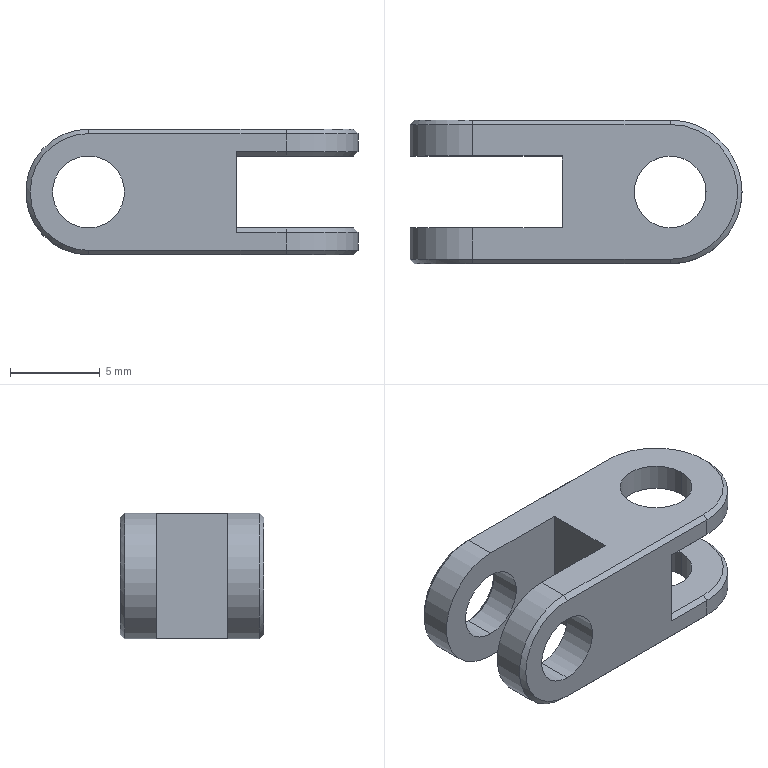Part | SolidWorks | features ICE 3, Chamfer 1, Extrusion 1, Scale 1 | 1 solid | 43 faces | box 18.5 x 8 x 7 mm | volume 447.364 mm3 | plane 19 | cylinder 14 | cone 10 | commonest cylinder face diameters 4 x8 8 x4 7 x2
STEP:
#1=CARTESIAN_POINT('',(14.75,4.,-3.5));
#2=VERTEX_POINT('',#1);
#3=CARTESIAN_POINT('',(11.,0.25,-3.5));
#4=VERTEX_POINT('',#3);
#5=CARTESIAN_POINT('',(11.,4.,-3.5));
#6=DIRECTION('',(0.,0.,-1.));
#7=DIRECTION('',(1.,0.,0.));
#8=AXIS2_PLACEMENT_3D('',#5,#6,#7);
#9=CIRCLE('',#8,3.75);
#10=EDGE_CURVE('',#2,#4,#9,.T.);
#11=ORIENTED_EDGE('',*,*,#10,.F.);
#12=CARTESIAN_POINT('',(15.,4.,-3.25));
#13=VERTEX_POINT('',#12);
#14=CARTESIAN_POINT('',(15.,4.,-3.25));
#15=DIRECTION('',(0.7071,0.,0.7071));
#16=VECTOR('',#15,1000.);
#17=LINE('',#14,#16);
#18=EDGE_CURVE('',#2,#13,#17,.T.);
#19=ORIENTED_EDGE('',*,*,#18,.T.);
#20=CARTESIAN_POINT('',(11.,0.,-3.25));
#21=VERTEX_POINT('',#20);
#22=CARTESIAN_POINT('',(11.,4.,-3.25));
#23=DIRECTION('',(0.,0.,1.));
#24=DIRECTION('',(1.,0.,0.));
#25=AXIS2_PLACEMENT_3D('',#22,#23,#24);
#26=CIRCLE('',#25,4.);
#27=EDGE_CURVE('',#21,#13,#26,.T.);
#28=ORIENTED_EDGE('',*,*,#27,.F.);
#29=CARTESIAN_POINT('',(11.,0.25,-3.5));
#30=DIRECTION('',(0.,-0.7071,0.7071));
#31=VECTOR('',#30,1000.);
#32=LINE('',#29,#31);
#33=EDGE_CURVE('',#4,#21,#32,.T.);
#34=ORIENTED_EDGE('',*,*,#33,.F.);
#35=EDGE_LOOP('',(#11,#19,#28,#34));
#36=FACE_OUTER_BOUND('',#35,.T.);
#37=CARTESIAN_POINT('',(11.,4.,-3.25));
#38=DIRECTION('',(0.,0.,1.));
#39=DIRECTION('',(1.,0.,0.));
#40=AXIS2_PLACEMENT_3D('',#37,#38,#39);
#41=CONICAL_SURFACE('',#40,4.,0.7854);
#42=ADVANCED_FACE('',(#36),#41,.T.);
#43=CARTESIAN_POINT('',(14.75,4.,2.));
#44=VERTEX_POINT('',#43);
#45=CARTESIAN_POINT('',(11.,0.25,2.));
#46=VERTEX_POINT('',#45);
#47=CARTESIAN_POINT('',(11.,4.,2.));
#48=DIRECTION('',(0.,0.,-1.));
#49=DIRECTION('',(1.,0.,0.));
#50=AXIS2_PLACEMENT_3D('',#47,#48,#49);
#51=CIRCLE('',#50,3.75);
#52=EDGE_CURVE('',#44,#46,#51,.T.);
#53=ORIENTED_EDGE('',*,*,#52,.F.);
#54=CARTESIAN_POINT('',(15.,4.,2.25));
#55=VERTEX_POINT('',#54);
#56=CARTESIAN_POINT('',(15.,4.,2.25));
#57=DIRECTION('',(0.7071,0.,0.7071));
#58=VECTOR('',#57,1000.);
#59=LINE('',#56,#58);
#60=EDGE_CURVE('',#44,#55,#59,.T.);
#61=ORIENTED_EDGE('',*,*,#60,.T.);
#62=CARTESIAN_POINT('',(11.,0.,2.25));
#63=VERTEX_POINT('',#62);
#64=CARTESIAN_POINT('',(11.,4.,2.25));
#65=DIRECTION('',(0.,0.,1.));
#66=DIRECTION('',(1.,0.,0.));
#67=AXIS2_PLACEMENT_3D('',#64,#65,#66);
#68=CIRCLE('',#67,4.);
#69=EDGE_CURVE('',#63,#55,#68,.T.);
#70=ORIENTED_EDGE('',*,*,#69,.F.);
#71=CARTESIAN_POINT('',(11.,0.,2.25));
#72=DIRECTION('',(0.,0.7071,-0.7071));
#73=VECTOR('',#72,1000.);
#74=LINE('',#71,#73);
#75=EDGE_CURVE('',#63,#46,#74,.T.);
#76=ORIENTED_EDGE('',*,*,#75,.T.);
#77=EDGE_LOOP('',(#53,#61,#70,#76));
#78=FACE_OUTER_BOUND('',#77,.T.);
#79=CARTESIAN_POINT('',(11.,4.,2.25));
#80=DIRECTION('',(0.,0.,1.));
#81=DIRECTION('',(1.,0.,0.));
#82=AXIS2_PLACEMENT_3D('',#79,#80,#81);
#83=CONICAL_SURFACE('',#82,4.,0.7854);
#84=ADVANCED_FACE('',(#78),#83,.T.);
#85=CARTESIAN_POINT('',(0.,7.75,-2.));
#86=VERTEX_POINT('',#85);
#87=CARTESIAN_POINT('',(0.,7.75,2.));
#88=VERTEX_POINT('',#87);
#89=CARTESIAN_POINT('',(0.,7.75,0.));
#90=DIRECTION('',(0.,1.,0.));
#91=DIRECTION('',(0.,0.,1.));
#92=AXIS2_PLACEMENT_3D('',#89,#90,#91);
#93=CIRCLE('',#92,2.);
#94=EDGE_CURVE('',#86,#88,#93,.T.);
#95=ORIENTED_EDGE('',*,*,#94,.F.);
#96=CARTESIAN_POINT('',(0.,8.,-2.25));
#97=VERTEX_POINT('',#96);
#98=CARTESIAN_POINT('',(0.,7.75,-2.));
#99=DIRECTION('',(0.,0.7071,-0.7071));
#100=VECTOR('',#99,1000.);
#101=LINE('',#98,#100);
#102=EDGE_CURVE('',#86,#97,#101,.T.);
#103=ORIENTED_EDGE('',*,*,#102,.T.);
#104=CARTESIAN_POINT('',(0.,8.,2.25));
#105=VERTEX_POINT('',#104);
#106=CARTESIAN_POINT('',(0.,8.,0.));
#107=DIRECTION('',(0.,-1.,0.));
#108=DIRECTION('',(0.,0.,1.));
#109=AXIS2_PLACEMENT_3D('',#106,#107,#108);
#110=CIRCLE('',#109,2.25);
#111=EDGE_CURVE('',#105,#97,#110,.T.);
#112=ORIENTED_EDGE('',*,*,#111,.F.);
#113=CARTESIAN_POINT('',(0.,7.75,2.));
#114=DIRECTION('',(0.,0.7071,0.7071));
#115=VECTOR('',#114,1000.);
#116=LINE('',#113,#115);
#117=EDGE_CURVE('',#88,#105,#116,.T.);
#118=ORIENTED_EDGE('',*,*,#117,.F.);
#119=EDGE_LOOP('',(#95,#103,#112,#118));
#120=FACE_OUTER_BOUND('',#119,.T.);
#121=CARTESIAN_POINT('',(0.,7.75,0.));
#122=DIRECTION('',(0.,1.,0.));
#123=DIRECTION('',(0.,0.,1.));
#124=AXIS2_PLACEMENT_3D('',#121,#122,#123);
#125=CONICAL_SURFACE('',#124,2.,0.7854);
#126=ADVANCED_FACE('',(#120),#125,.F.);
#127=CARTESIAN_POINT('',(9.,4.,2.));
#128=VERTEX_POINT('',#127);
#129=CARTESIAN_POINT('',(13.,4.,2.));
#130=VERTEX_POINT('',#129);
#131=CARTESIAN_POINT('',(11.,4.,2.));
#132=DIRECTION('',(0.,0.,1.));
#133=DIRECTION('',(1.,0.,0.));
#134=AXIS2_PLACEMENT_3D('',#131,#132,#133);
#135=CIRCLE('',#134,2.);
#136=EDGE_CURVE('',#128,#130,#135,.T.);
#137=ORIENTED_EDGE('',*,*,#136,.F.);
#138=CARTESIAN_POINT('',(9.,4.,3.5));
#139=VERTEX_POINT('',#138);
#140=CARTESIAN_POINT('',(9.,4.,-4.5));
#141=DIRECTION('',(0.,0.,1.));
#142=VECTOR('',#141,1000.);
#143=LINE('',#140,#142);
#144=EDGE_CURVE('',#128,#139,#143,.T.);
#145=ORIENTED_EDGE('',*,*,#144,.T.);
#146=CARTESIAN_POINT('',(13.,4.,3.5));
#147=VERTEX_POINT('',#146);
#148=CARTESIAN_POINT('',(11.,4.,3.5));
#149=DIRECTION('',(0.,0.,1.));
#150=DIRECTION('',(1.,0.,0.));
#151=AXIS2_PLACEMENT_3D('',#148,#149,#150);
#152=CIRCLE('',#151,2.);
#153=EDGE_CURVE('',#139,#147,#152,.T.);
#154=ORIENTED_EDGE('',*,*,#153,.T.);
#155=CARTESIAN_POINT('',(13.,4.,-4.5));
#156=DIRECTION('',(0.,0.,1.));
#157=VECTOR('',#156,1000.);
#158=LINE('',#155,#157);
#159=EDGE_CURVE('',#130,#147,#158,.T.);
#160=ORIENTED_EDGE('',*,*,#159,.F.);
#161=EDGE_LOOP('',(#137,#145,#154,#160));
#162=FACE_OUTER_BOUND('',#161,.T.);
#163=CARTESIAN_POINT('',(11.,4.,-4.5));
#164=DIRECTION('',(0.,0.,1.));
#165=DIRECTION('',(1.,0.,0.));
#166=AXIS2_PLACEMENT_3D('',#163,#164,#165);
#167=CYLINDRICAL_SURFACE('',#166,2.);
#168=ADVANCED_FACE('',(#162),#167,.F.);
#169=CARTESIAN_POINT('',(9.,4.,-3.5));
#170=VERTEX_POINT('',#169);
#171=CARTESIAN_POINT('',(13.,4.,-3.5));
#172=VERTEX_POINT('',#171);
#173=CARTESIAN_POINT('',(11.,4.,-3.5));
#174=DIRECTION('',(0.,0.,1.));
#175=DIRECTION('',(1.,0.,0.));
#176=AXIS2_PLACEMENT_3D('',#173,#174,#175);
#177=CIRCLE('',#176,2.);
#178=EDGE_CURVE('',#170,#172,#177,.T.);
#179=ORIENTED_EDGE('',*,*,#178,.F.);
#180=CARTESIAN_POINT('',(9.,4.,-2.));
#181=VERTEX_POINT('',#180);
#182=CARTESIAN_POINT('',(9.,4.,-4.5));
#183=DIRECTION('',(0.,0.,1.));
#184=VECTOR('',#183,1000.);
#185=LINE('',#182,#184);
#186=EDGE_CURVE('',#170,#181,#185,.T.);
#187=ORIENTED_EDGE('',*,*,#186,.T.);
#188=CARTESIAN_POINT('',(13.,4.,-2.));
#189=VERTEX_POINT('',#188);
#190=CARTESIAN_POINT('',(11.,4.,-2.));
#191=DIRECTION('',(0.,0.,-1.));
#192=DIRECTION('',(-1.,0.,0.));
#193=AXIS2_PLACEMENT_3D('',#190,#191,#192);
#194=CIRCLE('',#193,2.);
#195=EDGE_CURVE('',#189,#181,#194,.T.);
#196=ORIENTED_EDGE('',*,*,#195,.F.);
#197=CARTESIAN_POINT('',(13.,4.,-4.5));
#198=DIRECTION('',(0.,0.,1.));
#199=VECTOR('',#198,1000.);
#200=LINE('',#197,#199);
#201=EDGE_CURVE('',#172,#189,#200,.T.);
#202=ORIENTED_EDGE('',*,*,#201,.F.);
#203=EDGE_LOOP('',(#179,#187,#196,#202));
#204=FACE_OUTER_BOUND('',#203,.T.);
#205=CARTESIAN_POINT('',(11.,4.,-4.5));
#206=DIRECTION('',(0.,0.,1.));
#207=DIRECTION('',(1.,0.,0.));
#208=AXIS2_PLACEMENT_3D('',#205,#206,#207);
#209=CYLINDRICAL_SURFACE('',#208,2.);
#210=ADVANCED_FACE('',(#204),#209,.F.);
#211=ORIENTED_EDGE('',*,*,#69,.T.);
#212=CARTESIAN_POINT('',(15.,4.,3.25));
#213=VERTEX_POINT('',#212);
#214=CARTESIAN_POINT('',(15.,4.,-4.5));
#215=DIRECTION('',(0.,0.,1.));
#216=VECTOR('',#215,1000.);
#217=LINE('',#214,#216);
#218=EDGE_CURVE('',#55,#213,#217,.T.);
#219=ORIENTED_EDGE('',*,*,#218,.T.);
#220=CARTESIAN_POINT('',(11.,0.,3.25));
#221=VERTEX_POINT('',#220);
#222=CARTESIAN_POINT('',(11.,4.,3.25));
#223=DIRECTION('',(0.,0.,-1.));
#224=DIRECTION('',(-1.,0.,0.));
#225=AXIS2_PLACEMENT_3D('',#222,#223,#224);
#226=CIRCLE('',#225,4.);
#227=EDGE_CURVE('',#213,#221,#226,.T.);
#228=ORIENTED_EDGE('',*,*,#227,.T.);
#229=CARTESIAN_POINT('',(11.,0.,-4.5));
#230=DIRECTION('',(0.,0.,1.));
#231=VECTOR('',#230,1000.);
#232=LINE('',#229,#231);
#233=EDGE_CURVE('',#63,#221,#232,.T.);
#234=ORIENTED_EDGE('',*,*,#233,.F.);
#235=EDGE_LOOP('',(#211,#219,#228,#234));
#236=FACE_OUTER_BOUND('',#235,.T.);
#237=CARTESIAN_POINT('',(11.,4.,-4.5));
#238=DIRECTION('',(0.,0.,1.));
#239=DIRECTION('',(1.,0.,0.));
#240=AXIS2_PLACEMENT_3D('',#237,#238,#239);
#241=CYLINDRICAL_SURFACE('',#240,4.);
#242=ADVANCED_FACE('',(#236),#241,.T.);
#243=ORIENTED_EDGE('',*,*,#27,.T.);
#244=CARTESIAN_POINT('',(15.,4.,-2.25));
#245=VERTEX_POINT('',#244);
#246=CARTESIAN_POINT('',(15.,4.,-4.5));
#247=DIRECTION('',(0.,0.,1.));
#248=VECTOR('',#247,1000.);
#249=LINE('',#246,#248);
#250=EDGE_CURVE('',#13,#245,#249,.T.);
#251=ORIENTED_EDGE('',*,*,#250,.T.);
#252=CARTESIAN_POINT('',(11.,0.,-2.25));
#253=VERTEX_POINT('',#252);
#254=CARTESIAN_POINT('',(11.,4.,-2.25));
#255=DIRECTION('',(0.,0.,-1.));
#256=DIRECTION('',(-1.,0.,0.));
#257=AXIS2_PLACEMENT_3D('',#254,#255,#256);
#258=CIRCLE('',#257,4.);
#259=EDGE_CURVE('',#245,#253,#258,.T.);
#260=ORIENTED_EDGE('',*,*,#259,.T.);
#261=CARTESIAN_POINT('',(11.,0.,-4.5));
#262=DIRECTION('',(0.,0.,1.));
#263=VECTOR('',#262,1000.);
#264=LINE('',#261,#263);
#265=EDGE_CURVE('',#21,#253,#264,.T.);
#266=ORIENTED_EDGE('',*,*,#265,.F.);
#267=EDGE_LOOP('',(#243,#251,#260,#266));
#268=FACE_OUTER_BOUND('',#267,.T.);
#269=CARTESIAN_POINT('',(11.,4.,-4.5));
#270=DIRECTION('',(0.,0.,1.));
#271=DIRECTION('',(1.,0.,0.));
#272=AXIS2_PLACEMENT_3D('',#269,#270,#271);
#273=CYLINDRICAL_SURFACE('',#272,4.);
#274=ADVANCED_FACE('',(#268),#273,.T.);
#275=ORIENTED_EDGE('',*,*,#94,.T.);
#276=CARTESIAN_POINT('',(0.,6.,2.));
#277=VERTEX_POINT('',#276);
#278=CARTESIAN_POINT('',(0.,8.,2.));
#279=DIRECTION('',(0.,-1.,0.));
#280=VECTOR('',#279,1000.);
#281=LINE('',#278,#280);
#282=EDGE_CURVE('',#88,#277,#281,.T.);
#283=ORIENTED_EDGE('',*,*,#282,.T.);
#284=CARTESIAN_POINT('',(0.,6.,-2.));
#285=VERTEX_POINT('',#284);
#286=CARTESIAN_POINT('',(0.,6.,0.));
#287=DIRECTION('',(0.,-1.,0.));
#288=DIRECTION('',(0.,0.,-1.));
#289=AXIS2_PLACEMENT_3D('',#286,#287,#288);
#290=CIRCLE('',#289,2.);
#291=EDGE_CURVE('',#277,#285,#290,.T.);
#292=ORIENTED_EDGE('',*,*,#291,.T.);
#293=CARTESIAN_POINT('',(0.,8.,-2.));
#294=DIRECTION('',(0.,-1.,0.));
#295=VECTOR('',#294,1000.);
#296=LINE('',#293,#295);
#297=EDGE_CURVE('',#86,#285,#296,.T.);
#298=ORIENTED_EDGE('',*,*,#297,.F.);
#299=EDGE_LOOP('',(#275,#283,#292,#298));
#300=FACE_OUTER_BOUND('',#299,.T.);
#301=CARTESIAN_POINT('',(0.,8.,0.));
#302=DIRECTION('',(0.,-1.,0.));
#303=DIRECTION('',(0.,0.,-1.));
#304=AXIS2_PLACEMENT_3D('',#301,#302,#303);
#305=CYLINDRICAL_SURFACE('',#304,2.);
#306=ADVANCED_FACE('',(#300),#305,.F.);
#307=CARTESIAN_POINT('',(0.,2.,-2.));
#308=VERTEX_POINT('',#307);
#309=CARTESIAN_POINT('',(0.,2.,2.));
#310=VERTEX_POINT('',#309);
#311=CARTESIAN_POINT('',(0.,2.,0.));
#312=DIRECTION('',(0.,1.,0.));
#313=DIRECTION('',(0.,0.,1.));
#314=AXIS2_PLACEMENT_3D('',#311,#312,#313);
#315=CIRCLE('',#314,2.);
#316=EDGE_CURVE('',#308,#310,#315,.T.);
#317=ORIENTED_EDGE('',*,*,#316,.T.);
#318=CARTESIAN_POINT('',(0.,0.,2.));
#319=VERTEX_POINT('',#318);
#320=CARTESIAN_POINT('',(0.,8.,2.));
#321=DIRECTION('',(0.,-1.,0.));
#322=VECTOR('',#321,1000.);
#323=LINE('',#320,#322);
#324=EDGE_CURVE('',#310,#319,#323,.T.);
#325=ORIENTED_EDGE('',*,*,#324,.T.);
#326=CARTESIAN_POINT('',(0.,0.,-2.));
#327=VERTEX_POINT('',#326);
#328=CARTESIAN_POINT('',(0.,0.,0.));
#329=DIRECTION('',(0.,1.,0.));
#330=DIRECTION('',(0.,0.,1.));
#331=AXIS2_PLACEMENT_3D('',#328,#329,#330);
#332=CIRCLE('',#331,2.);
#333=EDGE_CURVE('',#327,#319,#332,.T.);
#334=ORIENTED_EDGE('',*,*,#333,.F.);
#335=CARTESIAN_POINT('',(0.,8.,-2.));
#336=DIRECTION('',(0.,-1.,0.));
#337=VECTOR('',#336,1000.);
#338=LINE('',#335,#337);
#339=EDGE_CURVE('',#308,#327,#338,.T.);
#340=ORIENTED_EDGE('',*,*,#339,.F.);
#341=EDGE_LOOP('',(#317,#325,#334,#340));
#342=FACE_OUTER_BOUND('',#341,.T.);
#343=CARTESIAN_POINT('',(0.,8.,0.));
#344=DIRECTION('',(0.,-1.,0.));
#345=DIRECTION('',(0.,0.,-1.));
#346=AXIS2_PLACEMENT_3D('',#343,#344,#345);
#347=CYLINDRICAL_SURFACE('',#346,2.);
#348=ADVANCED_FACE('',(#342),#347,.F.);
#349=CARTESIAN_POINT('',(11.,4.,3.5));
#350=DIRECTION('',(0.,0.,1.));
#351=DIRECTION('',(1.,0.,0.));
#352=AXIS2_PLACEMENT_3D('',#349,#350,#351);
#353=CIRCLE('',#352,2.);
#354=EDGE_CURVE('',#147,#139,#353,.T.);
#355=ORIENTED_EDGE('',*,*,#354,.F.);
#356=ORIENTED_EDGE('',*,*,#153,.F.);
#357=EDGE_LOOP('',(#355,#356));
#358=FACE_BOUND('',#357,.T.);
#359=CARTESIAN_POINT('',(0.,2.,3.5));
#360=VERTEX_POINT('',#359);
#361=CARTESIAN_POINT('',(0.,0.25,3.5));
#362=VERTEX_POINT('',#361);
#363=CARTESIAN_POINT('',(0.,8.,3.5));
#364=DIRECTION('',(0.,-1.,0.));
#365=VECTOR('',#364,1000.);
#366=LINE('',#363,#365);
#367=EDGE_CURVE('',#360,#362,#366,.T.);
#368=ORIENTED_EDGE('',*,*,#367,.T.);
#369=CARTESIAN_POINT('',(11.,0.25,3.5));
#370=VERTEX_POINT('',#369);
#371=CARTESIAN_POINT('',(0.,0.25,3.5));
#372=DIRECTION('',(1.,0.,0.));
#373=VECTOR('',#372,1000.);
#374=LINE('',#371,#373);
#375=EDGE_CURVE('',#362,#370,#374,.T.);
#376=ORIENTED_EDGE('',*,*,#375,.T.);
#377=CARTESIAN_POINT('',(11.,7.75,3.5));
#378=VERTEX_POINT('',#377);
#379=CARTESIAN_POINT('',(11.,4.,3.5));
#380=DIRECTION('',(0.,0.,1.));
#381=DIRECTION('',(-1.,0.,0.));
#382=AXIS2_PLACEMENT_3D('',#379,#380,#381);
#383=CIRCLE('',#382,3.75);
#384=EDGE_CURVE('',#370,#378,#383,.T.);
#385=ORIENTED_EDGE('',*,*,#384,.T.);
#386=CARTESIAN_POINT('',(0.,7.75,3.5));
#387=VERTEX_POINT('',#386);
#388=CARTESIAN_POINT('',(0.,7.75,3.5));
#389=DIRECTION('',(-1.,0.,0.));
#390=VECTOR('',#389,1000.);
#391=LINE('',#388,#390);
#392=EDGE_CURVE('',#378,#387,#391,.T.);
#393=ORIENTED_EDGE('',*,*,#392,.T.);
#394=CARTESIAN_POINT('',(0.,6.,3.5));
#395=VERTEX_POINT('',#394);
#396=CARTESIAN_POINT('',(0.,8.,3.5));
#397=DIRECTION('',(0.,-1.,0.));
#398=VECTOR('',#397,1000.);
#399=LINE('',#396,#398);
#400=EDGE_CURVE('',#387,#395,#399,.T.);
#401=ORIENTED_EDGE('',*,*,#400,.T.);
#402=CARTESIAN_POINT('',(5.,6.,3.5));
#403=VERTEX_POINT('',#402);
#404=CARTESIAN_POINT('',(5.,6.,3.5));
#405=DIRECTION('',(-1.,0.,0.));
#406=VECTOR('',#405,1000.);
#407=LINE('',#404,#406);
#408=EDGE_CURVE('',#403,#395,#407,.T.);
#409=ORIENTED_EDGE('',*,*,#408,.F.);
#410=CARTESIAN_POINT('',(5.,2.,3.5));
#411=VERTEX_POINT('',#410);
#412=CARTESIAN_POINT('',(5.,6.,3.5));
#413=DIRECTION('',(0.,-1.,0.));
#414=VECTOR('',#413,1000.);
#415=LINE('',#412,#414);
#416=EDGE_CURVE('',#403,#411,#415,.T.);
#417=ORIENTED_EDGE('',*,*,#416,.T.);
#418=CARTESIAN_POINT('',(5.,2.,3.5));
#419=DIRECTION('',(-1.,0.,0.));
#420=VECTOR('',#419,1000.);
#421=LINE('',#418,#420);
#422=EDGE_CURVE('',#411,#360,#421,.T.);
#423=ORIENTED_EDGE('',*,*,#422,.T.);
#424=EDGE_LOOP('',(#368,#376,#385,#393,#401,#409,#417,#423));
#425=FACE_OUTER_BOUND('',#424,.T.);
#426=CARTESIAN_POINT('',(0.,8.,3.5));
#427=DIRECTION('',(0.,0.,-1.));
#428=DIRECTION('',(-1.,0.,0.));
#429=AXIS2_PLACEMENT_3D('',#426,#427,#428);
#430=PLANE('',#429);
#431=ADVANCED_FACE('',(#358,#425),#430,.F.);
#432=CARTESIAN_POINT('',(11.,4.,-3.5));
#433=DIRECTION('',(0.,0.,1.));
#434=DIRECTION('',(1.,0.,0.));
#435=AXIS2_PLACEMENT_3D('',#432,#433,#434);
#436=CIRCLE('',#435,2.);
#437=EDGE_CURVE('',#172,#170,#436,.T.);
#438=ORIENTED_EDGE('',*,*,#437,.T.);
#439=ORIENTED_EDGE('',*,*,#178,.T.);
#440=EDGE_LOOP('',(#438,#439));
#441=FACE_BOUND('',#440,.T.);
#442=CARTESIAN_POINT('',(11.,7.75,-3.5));
#443=VERTEX_POINT('',#442);
#444=CARTESIAN_POINT('',(11.,4.,-3.5));
#445=DIRECTION('',(0.,0.,-1.));
#446=DIRECTION('',(1.,0.,0.));
#447=AXIS2_PLACEMENT_3D('',#444,#445,#446);
#448=CIRCLE('',#447,3.75);
#449=EDGE_CURVE('',#443,#2,#448,.T.);
#450=ORIENTED_EDGE('',*,*,#449,.T.);
#451=ORIENTED_EDGE('',*,*,#10,.T.);
#452=CARTESIAN_POINT('',(0.,0.25,-3.5));
#453=VERTEX_POINT('',#452);
#454=CARTESIAN_POINT('',(0.,0.25,-3.5));
#455=DIRECTION('',(-1.,0.,0.));
#456=VECTOR('',#455,1000.);
#457=LINE('',#454,#456);
#458=EDGE_CURVE('',#4,#453,#457,.T.);
#459=ORIENTED_EDGE('',*,*,#458,.T.);
#460=CARTESIAN_POINT('',(0.,2.,-3.5));
#461=VERTEX_POINT('',#460);
#462=CARTESIAN_POINT('',(0.,8.,-3.5));
#463=DIRECTION('',(0.,-1.,0.));
#464=VECTOR('',#463,1000.);
#465=LINE('',#462,#464);
#466=EDGE_CURVE('',#461,#453,#465,.T.);
#467=ORIENTED_EDGE('',*,*,#466,.F.);
#468=CARTESIAN_POINT('',(5.,2.,-3.5));
#469=VERTEX_POINT('',#468);
#470=CARTESIAN_POINT('',(5.,2.,-3.5));
#471=DIRECTION('',(-1.,0.,0.));
#472=VECTOR('',#471,1000.);
#473=LINE('',#470,#472);
#474=EDGE_CURVE('',#469,#461,#473,.T.);
#475=ORIENTED_EDGE('',*,*,#474,.F.);
#476=CARTESIAN_POINT('',(5.,6.,-3.5));
#477=VERTEX_POINT('',#476);
#478=CARTESIAN_POINT('',(5.,6.,-3.5));
#479=DIRECTION('',(0.,1.,0.));
#480=VECTOR('',#479,1000.);
#481=LINE('',#478,#480);
#482=EDGE_CURVE('',#469,#477,#481,.T.);
#483=ORIENTED_EDGE('',*,*,#482,.T.);
#484=CARTESIAN_POINT('',(0.,6.,-3.5));
#485=VERTEX_POINT('',#484);
#486=CARTESIAN_POINT('',(5.,6.,-3.5));
#487=DIRECTION('',(-1.,0.,0.));
#488=VECTOR('',#487,1000.);
#489=LINE('',#486,#488);
#490=EDGE_CURVE('',#477,#485,#489,.T.);
#491=ORIENTED_EDGE('',*,*,#490,.T.);
#492=CARTESIAN_POINT('',(0.,7.75,-3.5));
#493=VERTEX_POINT('',#492);
#494=CARTESIAN_POINT('',(0.,8.,-3.5));
#495=DIRECTION('',(0.,-1.,0.));
#496=VECTOR('',#495,1000.);
#497=LINE('',#494,#496);
#498=EDGE_CURVE('',#493,#485,#497,.T.);
#499=ORIENTED_EDGE('',*,*,#498,.F.);
#500=CARTESIAN_POINT('',(11.,7.75,-3.5));
#501=DIRECTION('',(1.,0.,0.));
#502=VECTOR('',#501,1000.);
#503=LINE('',#500,#502);
#504=EDGE_CURVE('',#493,#443,#503,.T.);
#505=ORIENTED_EDGE('',*,*,#504,.T.);
#506=EDGE_LOOP('',(#450,#451,#459,#467,#475,#483,#491,#499,#505));
#507=FACE_OUTER_BOUND('',#506,.T.);
#508=CARTESIAN_POINT('',(0.,8.,-3.5));
#509=DIRECTION('',(0.,0.,1.));
#510=DIRECTION('',(1.,0.,0.));
#511=AXIS2_PLACEMENT_3D('',#508,#509,#510);
#512=PLANE('',#511);
#513=ADVANCED_FACE('',(#441,#507),#512,.F.);
#514=ORIENTED_EDGE('',*,*,#466,.T.);
#515=CARTESIAN_POINT('',(0.,0.25,0.));
#516=DIRECTION('',(0.,1.,0.));
#517=DIRECTION('',(0.,0.,1.));
#518=AXIS2_PLACEMENT_3D('',#515,#516,#517);
#519=CIRCLE('',#518,3.5);
#520=EDGE_CURVE('',#453,#362,#519,.T.);
#521=ORIENTED_EDGE('',*,*,#520,.T.);
#522=ORIENTED_EDGE('',*,*,#367,.F.);
#523=CARTESIAN_POINT('',(0.,2.,0.));
#524=DIRECTION('',(0.,1.,0.));
#525=DIRECTION('',(0.,0.,1.));
#526=AXIS2_PLACEMENT_3D('',#523,#524,#525);
#527=CIRCLE('',#526,3.5);
#528=EDGE_CURVE('',#461,#360,#527,.T.);
#529=ORIENTED_EDGE('',*,*,#528,.F.);
#530=EDGE_LOOP('',(#514,#521,#522,#529));
#531=FACE_OUTER_BOUND('',#530,.T.);
#532=CARTESIAN_POINT('',(0.,8.,0.));
#533=DIRECTION('',(0.,-1.,0.));
#534=DIRECTION('',(0.,0.,-1.));
#535=AXIS2_PLACEMENT_3D('',#532,#533,#534);
#536=CYLINDRICAL_SURFACE('',#535,3.5);
#537=ADVANCED_FACE('',(#531),#536,.T.);
#538=ORIENTED_EDGE('',*,*,#400,.F.);
#539=CARTESIAN_POINT('',(0.,7.75,0.));
#540=DIRECTION('',(0.,-1.,0.));
#541=DIRECTION('',(0.,0.,1.));
#542=AXIS2_PLACEMENT_3D('',#539,#540,#541);
#543=CIRCLE('',#542,3.5);
#544=EDGE_CURVE('',#387,#493,#543,.T.);
#545=ORIENTED_EDGE('',*,*,#544,.T.);
#546=ORIENTED_EDGE('',*,*,#498,.T.);
#547=CARTESIAN_POINT('',(0.,6.,0.));
#548=DIRECTION('',(0.,-1.,0.));
#549=DIRECTION('',(0.,0.,-1.));
#550=AXIS2_PLACEMENT_3D('',#547,#548,#549);
#551=CIRCLE('',#550,3.5);
#552=EDGE_CURVE('',#395,#485,#551,.T.);
#553=ORIENTED_EDGE('',*,*,#552,.F.);
#554=EDGE_LOOP('',(#538,#545,#546,#553));
#555=FACE_OUTER_BOUND('',#554,.T.);
#556=CARTESIAN_POINT('',(0.,8.,0.));
#557=DIRECTION('',(0.,-1.,0.));
#558=DIRECTION('',(0.,0.,-1.));
#559=AXIS2_PLACEMENT_3D('',#556,#557,#558);
#560=CYLINDRICAL_SURFACE('',#559,3.5);
#561=ADVANCED_FACE('',(#555),#560,.T.);
#562=ORIENTED_EDGE('',*,*,#324,.F.);
#563=CARTESIAN_POINT('',(0.,2.,0.));
#564=DIRECTION('',(0.,1.,0.));
#565=DIRECTION('',(0.,0.,1.));
#566=AXIS2_PLACEMENT_3D('',#563,#564,#565);
#567=CIRCLE('',#566,2.);
#568=EDGE_CURVE('',#310,#308,#567,.T.);
#569=ORIENTED_EDGE('',*,*,#568,.T.);
#570=ORIENTED_EDGE('',*,*,#339,.T.);
#571=CARTESIAN_POINT('',(0.,0.,0.));
#572=DIRECTION('',(0.,1.,0.));
#573=DIRECTION('',(0.,0.,1.));
#574=AXIS2_PLACEMENT_3D('',#571,#572,#573);
#575=CIRCLE('',#574,2.);
#576=EDGE_CURVE('',#319,#327,#575,.T.);
#577=ORIENTED_EDGE('',*,*,#576,.F.);
#578=EDGE_LOOP('',(#562,#569,#570,#577));
#579=FACE_OUTER_BOUND('',#578,.T.);
#580=CARTESIAN_POINT('',(0.,8.,0.));
#581=DIRECTION('',(0.,-1.,0.));
#582=DIRECTION('',(0.,0.,-1.));
#583=AXIS2_PLACEMENT_3D('',#580,#581,#582);
#584=CYLINDRICAL_SURFACE('',#583,2.);
#585=ADVANCED_FACE('',(#579),#584,.F.);
#586=ORIENTED_EDGE('',*,*,#282,.F.);
#587=CARTESIAN_POINT('',(0.,7.75,0.));
#588=DIRECTION('',(0.,1.,0.));
#589=DIRECTION('',(0.,0.,1.));
#590=AXIS2_PLACEMENT_3D('',#587,#588,#589);
#591=CIRCLE('',#590,2.);
#592=EDGE_CURVE('',#88,#86,#591,.T.);
#593=ORIENTED_EDGE('',*,*,#592,.T.);
#594=ORIENTED_EDGE('',*,*,#297,.T.);
#595=CARTESIAN_POINT('',(0.,6.,0.));
#596=DIRECTION('',(0.,-1.,0.));
#597=DIRECTION('',(0.,0.,-1.));
#598=AXIS2_PLACEMENT_3D('',#595,#596,#597);
#599=CIRCLE('',#598,2.);
#600=EDGE_CURVE('',#285,#277,#599,.T.);
#601=ORIENTED_EDGE('',*,*,#600,.T.);
#602=EDGE_LOOP('',(#586,#593,#594,#601));
#603=FACE_OUTER_BOUND('',#602,.T.);
#604=CARTESIAN_POINT('',(0.,8.,0.));
#605=DIRECTION('',(0.,-1.,0.));
#606=DIRECTION('',(0.,0.,-1.));
#607=AXIS2_PLACEMENT_3D('',#604,#605,#606);
#608=CYLINDRICAL_SURFACE('',#607,2.);
#609=ADVANCED_FACE('',(#603),#608,.F.);
#610=CARTESIAN_POINT('',(11.,4.,2.));
#611=DIRECTION('',(0.,0.,1.));
#612=DIRECTION('',(1.,0.,0.));
#613=AXIS2_PLACEMENT_3D('',#610,#611,#612);
#614=CIRCLE('',#613,2.);
#615=EDGE_CURVE('',#130,#128,#614,.T.);
#616=ORIENTED_EDGE('',*,*,#615,.T.);
#617=ORIENTED_EDGE('',*,*,#136,.T.);
#618=EDGE_LOOP('',(#616,#617));
#619=FACE_BOUND('',#618,.T.);
#620=CARTESIAN_POINT('',(11.,7.75,2.));
#621=VERTEX_POINT('',#620);
#622=CARTESIAN_POINT('',(11.,4.,2.));
#623=DIRECTION('',(0.,0.,-1.));
#624=DIRECTION('',(1.,0.,0.));
#625=AXIS2_PLACEMENT_3D('',#622,#623,#624);
#626=CIRCLE('',#625,3.75);
#627=EDGE_CURVE('',#621,#44,#626,.T.);
#628=ORIENTED_EDGE('',*,*,#627,.T.);
#629=ORIENTED_EDGE('',*,*,#52,.T.);
#630=CARTESIAN_POINT('',(8.232,0.25,2.));
#631=VERTEX_POINT('',#630);
#632=CARTESIAN_POINT('',(15.,0.25,2.));
#633=DIRECTION('',(-1.,0.,0.));
#634=VECTOR('',#633,1000.);
#635=LINE('',#632,#634);
#636=EDGE_CURVE('',#46,#631,#635,.T.);
#637=ORIENTED_EDGE('',*,*,#636,.T.);
#638=CARTESIAN_POINT('',(8.232,7.75,2.));
#639=VERTEX_POINT('',#638);
#640=CARTESIAN_POINT('',(8.232,0.,2.));
#641=DIRECTION('',(0.,1.,0.));
#642=VECTOR('',#641,1000.);
#643=LINE('',#640,#642);
#644=EDGE_CURVE('',#631,#639,#643,.T.);
#645=ORIENTED_EDGE('',*,*,#644,.T.);
#646=CARTESIAN_POINT('',(11.,7.75,2.));
#647=DIRECTION('',(1.,0.,0.));
#648=VECTOR('',#647,1000.);
#649=LINE('',#646,#648);
#650=EDGE_CURVE('',#639,#621,#649,.T.);
#651=ORIENTED_EDGE('',*,*,#650,.T.);
#652=EDGE_LOOP('',(#628,#629,#637,#645,#651));
#653=FACE_OUTER_BOUND('',#652,.T.);
#654=CARTESIAN_POINT('',(15.,0.,2.));
#655=DIRECTION('',(0.,0.,1.));
#656=DIRECTION('',(1.,0.,0.));
#657=AXIS2_PLACEMENT_3D('',#654,#655,#656);
#658=PLANE('',#657);
#659=ADVANCED_FACE('',(#619,#653),#658,.F.);
#660=ORIENTED_EDGE('',*,*,#195,.T.);
#661=CARTESIAN_POINT('',(11.,4.,-2.));
#662=DIRECTION('',(0.,0.,-1.));
#663=DIRECTION('',(-1.,0.,0.));
#664=AXIS2_PLACEMENT_3D('',#661,#662,#663);
#665=CIRCLE('',#664,2.);
#666=EDGE_CURVE('',#181,#189,#665,.T.);
#667=ORIENTED_EDGE('',*,*,#666,.T.);
#668=EDGE_LOOP('',(#660,#667));
#669=FACE_BOUND('',#668,.T.);
#670=CARTESIAN_POINT('',(8.232,0.25,-2.));
#671=VERTEX_POINT('',#670);
#672=CARTESIAN_POINT('',(8.232,7.75,-2.));
#673=VERTEX_POINT('',#672);
#674=CARTESIAN_POINT('',(8.232,0.,-2.));
#675=DIRECTION('',(0.,1.,0.));
#676=VECTOR('',#675,1000.);
#677=LINE('',#674,#676);
#678=EDGE_CURVE('',#671,#673,#677,.T.);
#679=ORIENTED_EDGE('',*,*,#678,.F.);
#680=CARTESIAN_POINT('',(11.,0.25,-2.));
#681=VERTEX_POINT('',#680);
#682=CARTESIAN_POINT('',(15.,0.25,-2.));
#683=DIRECTION('',(1.,0.,0.));
#684=VECTOR('',#683,1000.);
#685=LINE('',#682,#684);
#686=EDGE_CURVE('',#671,#681,#685,.T.);
#687=ORIENTED_EDGE('',*,*,#686,.T.);
#688=CARTESIAN_POINT('',(11.,7.75,-2.));
#689=VERTEX_POINT('',#688);
#690=CARTESIAN_POINT('',(11.,4.,-2.));
#691=DIRECTION('',(0.,0.,1.));
#692=DIRECTION('',(-1.,0.,0.));
#693=AXIS2_PLACEMENT_3D('',#690,#691,#692);
#694=CIRCLE('',#693,3.75);
#695=EDGE_CURVE('',#681,#689,#694,.T.);
#696=ORIENTED_EDGE('',*,*,#695,.T.);
#697=CARTESIAN_POINT('',(8.232,7.75,-2.));
#698=DIRECTION('',(-1.,0.,0.));
#699=VECTOR('',#698,1000.);
#700=LINE('',#697,#699);
#701=EDGE_CURVE('',#689,#673,#700,.T.);
#702=ORIENTED_EDGE('',*,*,#701,.T.);
#703=EDGE_LOOP('',(#679,#687,#696,#702));
#704=FACE_OUTER_BOUND('',#703,.T.);
#705=CARTESIAN_POINT('',(15.,0.,-2.));
#706=DIRECTION('',(0.,0.,-1.));
#707=DIRECTION('',(-1.,0.,0.));
#708=AXIS2_PLACEMENT_3D('',#705,#706,#707);
#709=PLANE('',#708);
#710=ADVANCED_FACE('',(#669,#704),#709,.F.);
#711=ORIENTED_EDGE('',*,*,#111,.T.);
#712=CARTESIAN_POINT('',(0.,8.,0.));
#713=DIRECTION('',(0.,-1.,0.));
#714=DIRECTION('',(0.,0.,1.));
#715=AXIS2_PLACEMENT_3D('',#712,#713,#714);
#716=CIRCLE('',#715,2.25);
#717=EDGE_CURVE('',#97,#105,#716,.T.);
#718=ORIENTED_EDGE('',*,*,#717,.T.);
#719=EDGE_LOOP('',(#711,#718));
#720=FACE_BOUND('',#719,.T.);
#721=CARTESIAN_POINT('',(7.982,8.,2.25));
#722=VERTEX_POINT('',#721);
#723=CARTESIAN_POINT('',(7.982,8.,-2.25));
#724=VERTEX_POINT('',#723);
#725=CARTESIAN_POINT('',(7.982,8.,-2.));
#726=DIRECTION('',(0.,0.,-1.));
#727=VECTOR('',#726,1000.);
#728=LINE('',#725,#727);
#729=EDGE_CURVE('',#722,#724,#728,.T.);
#730=ORIENTED_EDGE('',*,*,#729,.T.);
#731=CARTESIAN_POINT('',(11.,8.,-2.25));
#732=VERTEX_POINT('',#731);
#733=CARTESIAN_POINT('',(11.,8.,-2.25));
#734=DIRECTION('',(1.,0.,0.));
#735=VECTOR('',#734,1000.);
#736=LINE('',#733,#735);
#737=EDGE_CURVE('',#724,#732,#736,.T.);
#738=ORIENTED_EDGE('',*,*,#737,.T.);
#739=CARTESIAN_POINT('',(11.,8.,-3.25));
#740=VERTEX_POINT('',#739);
#741=CARTESIAN_POINT('',(11.,8.,-4.5));
#742=DIRECTION('',(0.,0.,1.));
#743=VECTOR('',#742,1000.);
#744=LINE('',#741,#743);
#745=EDGE_CURVE('',#740,#732,#744,.T.);
#746=ORIENTED_EDGE('',*,*,#745,.F.);
#747=CARTESIAN_POINT('',(0.,8.,-3.25));
#748=VERTEX_POINT('',#747);
#749=CARTESIAN_POINT('',(0.,8.,-3.25));
#750=DIRECTION('',(-1.,0.,0.));
#751=VECTOR('',#750,1000.);
#752=LINE('',#749,#751);
#753=EDGE_CURVE('',#740,#748,#752,.T.);
#754=ORIENTED_EDGE('',*,*,#753,.T.);
#755=CARTESIAN_POINT('',(0.,8.,3.25));
#756=VERTEX_POINT('',#755);
#757=CARTESIAN_POINT('',(0.,8.,0.));
#758=DIRECTION('',(0.,1.,0.));
#759=DIRECTION('',(0.,0.,1.));
#760=AXIS2_PLACEMENT_3D('',#757,#758,#759);
#761=CIRCLE('',#760,3.25);
#762=EDGE_CURVE('',#748,#756,#761,.T.);
#763=ORIENTED_EDGE('',*,*,#762,.T.);
#764=CARTESIAN_POINT('',(11.,8.,3.25));
#765=VERTEX_POINT('',#764);
#766=CARTESIAN_POINT('',(11.,8.,3.25));
#767=DIRECTION('',(1.,0.,0.));
#768=VECTOR('',#767,1000.);
#769=LINE('',#766,#768);
#770=EDGE_CURVE('',#756,#765,#769,.T.);
#771=ORIENTED_EDGE('',*,*,#770,.T.);
#772=CARTESIAN_POINT('',(11.,8.,2.25));
#773=VERTEX_POINT('',#772);
#774=CARTESIAN_POINT('',(11.,8.,-4.5));
#775=DIRECTION('',(0.,0.,1.));
#776=VECTOR('',#775,1000.);
#777=LINE('',#774,#776);
#778=EDGE_CURVE('',#773,#765,#777,.T.);
#779=ORIENTED_EDGE('',*,*,#778,.F.);
#780=CARTESIAN_POINT('',(8.232,8.,2.25));
#781=DIRECTION('',(-1.,0.,0.));
#782=VECTOR('',#781,1000.);
#783=LINE('',#780,#782);
#784=EDGE_CURVE('',#773,#722,#783,.T.);
#785=ORIENTED_EDGE('',*,*,#784,.T.);
#786=EDGE_LOOP('',(#730,#738,#746,#754,#763,#771,#779,#785));
#787=FACE_OUTER_BOUND('',#786,.T.);
#788=CARTESIAN_POINT('',(0.,8.,0.));
#789=DIRECTION('',(0.,1.,0.));
#790=DIRECTION('',(0.,0.,1.));
#791=AXIS2_PLACEMENT_3D('',#788,#789,#790);
#792=PLANE('',#791);
#793=ADVANCED_FACE('',(#720,#787),#792,.T.);
#794=ORIENTED_EDGE('',*,*,#265,.T.);
#795=CARTESIAN_POINT('',(8.232,0.,-2.25));
#796=VERTEX_POINT('',#795);
#797=CARTESIAN_POINT('',(0.,0.,-2.25));
#798=DIRECTION('',(-1.,0.,0.));
#799=VECTOR('',#798,1000.);
#800=LINE('',#797,#799);
#801=EDGE_CURVE('',#253,#796,#800,.T.);
#802=ORIENTED_EDGE('',*,*,#801,.T.);
#803=CARTESIAN_POINT('',(8.232,0.,2.25));
#804=VERTEX_POINT('',#803);
#805=CARTESIAN_POINT('',(8.232,0.,-2.));
#806=DIRECTION('',(0.,0.,1.));
#807=VECTOR('',#806,1000.);
#808=LINE('',#805,#807);
#809=EDGE_CURVE('',#796,#804,#808,.T.);
#810=ORIENTED_EDGE('',*,*,#809,.T.);
#811=CARTESIAN_POINT('',(0.,0.,2.25));
#812=DIRECTION('',(1.,0.,0.));
#813=VECTOR('',#812,1000.);
#814=LINE('',#811,#813);
#815=EDGE_CURVE('',#804,#63,#814,.T.);
#816=ORIENTED_EDGE('',*,*,#815,.T.);
#817=ORIENTED_EDGE('',*,*,#233,.T.);
#818=CARTESIAN_POINT('',(0.,0.,3.25));
#819=VERTEX_POINT('',#818);
#820=CARTESIAN_POINT('',(0.,0.,3.25));
#821=DIRECTION('',(-1.,0.,0.));
#822=VECTOR('',#821,1000.);
#823=LINE('',#820,#822);
#824=EDGE_CURVE('',#221,#819,#823,.T.);
#825=ORIENTED_EDGE('',*,*,#824,.T.);
#826=CARTESIAN_POINT('',(0.,0.,-3.25));
#827=VERTEX_POINT('',#826);
#828=CARTESIAN_POINT('',(0.,0.,0.));
#829=DIRECTION('',(0.,-1.,0.));
#830=DIRECTION('',(0.,0.,1.));
#831=AXIS2_PLACEMENT_3D('',#828,#829,#830);
#832=CIRCLE('',#831,3.25);
#833=EDGE_CURVE('',#819,#827,#832,.T.);
#834=ORIENTED_EDGE('',*,*,#833,.T.);
#835=CARTESIAN_POINT('',(0.,0.,-3.25));
#836=DIRECTION('',(1.,0.,0.));
#837=VECTOR('',#836,1000.);
#838=LINE('',#835,#837);
#839=EDGE_CURVE('',#827,#21,#838,.T.);
#840=ORIENTED_EDGE('',*,*,#839,.T.);
#841=EDGE_LOOP('',(#794,#802,#810,#816,#817,#825,#834,#840));
#842=FACE_OUTER_BOUND('',#841,.T.);
#843=ORIENTED_EDGE('',*,*,#333,.T.);
#844=ORIENTED_EDGE('',*,*,#576,.T.);
#845=EDGE_LOOP('',(#843,#844));
#846=FACE_BOUND('',#845,.T.);
#847=CARTESIAN_POINT('',(0.,0.,0.));
#848=DIRECTION('',(0.,1.,0.));
#849=DIRECTION('',(0.,0.,1.));
#850=AXIS2_PLACEMENT_3D('',#847,#848,#849);
#851=PLANE('',#850);
#852=ADVANCED_FACE('',(#842,#846),#851,.F.);
#853=ORIENTED_EDGE('',*,*,#678,.T.);
#854=CARTESIAN_POINT('',(8.232,7.75,2.));
#855=DIRECTION('',(0.,0.,1.));
#856=VECTOR('',#855,1000.);
#857=LINE('',#854,#856);
#858=EDGE_CURVE('',#673,#639,#857,.T.);
#859=ORIENTED_EDGE('',*,*,#858,.T.);
#860=ORIENTED_EDGE('',*,*,#644,.F.);
#861=CARTESIAN_POINT('',(8.232,2.125,0.125));
#862=DIRECTION('',(0.,-0.7071,0.7071));
#863=VECTOR('',#862,1000.);
#864=LINE('',#861,#863);
#865=EDGE_CURVE('',#631,#804,#864,.T.);
#866=ORIENTED_EDGE('',*,*,#865,.T.);
#867=ORIENTED_EDGE('',*,*,#809,.F.);
#868=CARTESIAN_POINT('',(8.232,0.125,-2.125));
#869=DIRECTION('',(0.,0.7071,0.7071));
#870=VECTOR('',#869,1000.);
#871=LINE('',#868,#870);
#872=EDGE_CURVE('',#796,#671,#871,.T.);
#873=ORIENTED_EDGE('',*,*,#872,.T.);
#874=EDGE_LOOP('',(#853,#859,#860,#866,#867,#873));
#875=FACE_OUTER_BOUND('',#874,.T.);
#876=CARTESIAN_POINT('',(8.232,0.,-2.));
#877=DIRECTION('',(-1.,0.,0.));
#878=DIRECTION('',(0.,0.,1.));
#879=AXIS2_PLACEMENT_3D('',#876,#877,#878);
#880=PLANE('',#879);
#881=ADVANCED_FACE('',(#875),#880,.F.);
#882=ORIENTED_EDGE('',*,*,#250,.F.);
#883=CARTESIAN_POINT('',(11.,4.,-3.25));
#884=DIRECTION('',(0.,0.,1.));
#885=DIRECTION('',(1.,0.,0.));
#886=AXIS2_PLACEMENT_3D('',#883,#884,#885);
#887=CIRCLE('',#886,4.);
#888=EDGE_CURVE('',#13,#740,#887,.T.);
#889=ORIENTED_EDGE('',*,*,#888,.T.);
#890=ORIENTED_EDGE('',*,*,#745,.T.);
#891=CARTESIAN_POINT('',(11.,4.,-2.25));
#892=DIRECTION('',(0.,0.,-1.));
#893=DIRECTION('',(-1.,0.,0.));
#894=AXIS2_PLACEMENT_3D('',#891,#892,#893);
#895=CIRCLE('',#894,4.);
#896=EDGE_CURVE('',#732,#245,#895,.T.);
#897=ORIENTED_EDGE('',*,*,#896,.T.);
#898=EDGE_LOOP('',(#882,#889,#890,#897));
#899=FACE_OUTER_BOUND('',#898,.T.);
#900=CARTESIAN_POINT('',(11.,4.,-4.5));
#901=DIRECTION('',(0.,0.,1.));
#902=DIRECTION('',(1.,0.,0.));
#903=AXIS2_PLACEMENT_3D('',#900,#901,#902);
#904=CYLINDRICAL_SURFACE('',#903,4.);
#905=ADVANCED_FACE('',(#899),#904,.T.);
#906=ORIENTED_EDGE('',*,*,#218,.F.);
#907=CARTESIAN_POINT('',(11.,4.,2.25));
#908=DIRECTION('',(0.,0.,1.));
#909=DIRECTION('',(1.,0.,0.));
#910=AXIS2_PLACEMENT_3D('',#907,#908,#909);
#911=CIRCLE('',#910,4.);
#912=EDGE_CURVE('',#55,#773,#911,.T.);
#913=ORIENTED_EDGE('',*,*,#912,.T.);
#914=ORIENTED_EDGE('',*,*,#778,.T.);
#915=CARTESIAN_POINT('',(11.,4.,3.25));
#916=DIRECTION('',(0.,0.,-1.));
#917=DIRECTION('',(-1.,0.,0.));
#918=AXIS2_PLACEMENT_3D('',#915,#916,#917);
#919=CIRCLE('',#918,4.);
#920=EDGE_CURVE('',#765,#213,#919,.T.);
#921=ORIENTED_EDGE('',*,*,#920,.T.);
#922=EDGE_LOOP('',(#906,#913,#914,#921));
#923=FACE_OUTER_BOUND('',#922,.T.);
#924=CARTESIAN_POINT('',(11.,4.,-4.5));
#925=DIRECTION('',(0.,0.,1.));
#926=DIRECTION('',(1.,0.,0.));
#927=AXIS2_PLACEMENT_3D('',#924,#925,#926);
#928=CYLINDRICAL_SURFACE('',#927,4.);
#929=ADVANCED_FACE('',(#923),#928,.T.);
#930=ORIENTED_EDGE('',*,*,#186,.F.);
#931=ORIENTED_EDGE('',*,*,#437,.F.);
#932=ORIENTED_EDGE('',*,*,#201,.T.);
#933=ORIENTED_EDGE('',*,*,#666,.F.);
#934=EDGE_LOOP('',(#930,#931,#932,#933));
#935=FACE_OUTER_BOUND('',#934,.T.);
#936=CARTESIAN_POINT('',(11.,4.,-4.5));
#937=DIRECTION('',(0.,0.,1.));
#938=DIRECTION('',(1.,0.,0.));
#939=AXIS2_PLACEMENT_3D('',#936,#937,#938);
#940=CYLINDRICAL_SURFACE('',#939,2.);
#941=ADVANCED_FACE('',(#935),#940,.F.);
#942=ORIENTED_EDGE('',*,*,#144,.F.);
#943=ORIENTED_EDGE('',*,*,#615,.F.);
#944=ORIENTED_EDGE('',*,*,#159,.T.);
#945=ORIENTED_EDGE('',*,*,#354,.T.);
#946=EDGE_LOOP('',(#942,#943,#944,#945));
#947=FACE_OUTER_BOUND('',#946,.T.);
#948=CARTESIAN_POINT('',(11.,4.,-4.5));
#949=DIRECTION('',(0.,0.,1.));
#950=DIRECTION('',(1.,0.,0.));
#951=AXIS2_PLACEMENT_3D('',#948,#949,#950);
#952=CYLINDRICAL_SURFACE('',#951,2.);
#953=ADVANCED_FACE('',(#947),#952,.F.);
#954=ORIENTED_EDGE('',*,*,#316,.F.);
#955=ORIENTED_EDGE('',*,*,#568,.F.);
#956=EDGE_LOOP('',(#954,#955));
#957=FACE_BOUND('',#956,.T.);
#958=ORIENTED_EDGE('',*,*,#528,.T.);
#959=ORIENTED_EDGE('',*,*,#422,.F.);
#960=CARTESIAN_POINT('',(5.,2.,3.5));
#961=DIRECTION('',(0.,0.,-1.));
#962=VECTOR('',#961,1000.);
#963=LINE('',#960,#962);
#964=EDGE_CURVE('',#411,#469,#963,.T.);
#965=ORIENTED_EDGE('',*,*,#964,.T.);
#966=ORIENTED_EDGE('',*,*,#474,.T.);
#967=EDGE_LOOP('',(#958,#959,#965,#966));
#968=FACE_OUTER_BOUND('',#967,.T.);
#969=CARTESIAN_POINT('',(5.,2.,3.5));
#970=DIRECTION('',(0.,1.,0.));
#971=DIRECTION('',(0.,0.,1.));
#972=AXIS2_PLACEMENT_3D('',#969,#970,#971);
#973=PLANE('',#972);
#974=ADVANCED_FACE('',(#957,#968),#973,.T.);
#975=ORIENTED_EDGE('',*,*,#600,.F.);
#976=ORIENTED_EDGE('',*,*,#291,.F.);
#977=EDGE_LOOP('',(#975,#976));
#978=FACE_BOUND('',#977,.T.);
#979=ORIENTED_EDGE('',*,*,#552,.T.);
#980=ORIENTED_EDGE('',*,*,#490,.F.);
#981=CARTESIAN_POINT('',(5.,6.,3.5));
#982=DIRECTION('',(0.,0.,1.));
#983=VECTOR('',#982,1000.);
#984=LINE('',#981,#983);
#985=EDGE_CURVE('',#477,#403,#984,.T.);
#986=ORIENTED_EDGE('',*,*,#985,.T.);
#987=ORIENTED_EDGE('',*,*,#408,.T.);
#988=EDGE_LOOP('',(#979,#980,#986,#987));
#989=FACE_OUTER_BOUND('',#988,.T.);
#990=CARTESIAN_POINT('',(5.,6.,3.5));
#991=DIRECTION('',(0.,-1.,0.));
#992=DIRECTION('',(0.,0.,-1.));
#993=AXIS2_PLACEMENT_3D('',#990,#991,#992);
#994=PLANE('',#993);
#995=ADVANCED_FACE('',(#978,#989),#994,.T.);
#996=ORIENTED_EDGE('',*,*,#416,.F.);
#997=ORIENTED_EDGE('',*,*,#985,.F.);
#998=ORIENTED_EDGE('',*,*,#482,.F.);
#999=ORIENTED_EDGE('',*,*,#964,.F.);
#1000=EDGE_LOOP('',(#996,#997,#998,#999));
#1001=FACE_OUTER_BOUND('',#1000,.T.);
#1002=CARTESIAN_POINT('',(5.,0.,0.));
#1003=DIRECTION('',(1.,0.,0.));
#1004=DIRECTION('',(0.,0.,-1.));
#1005=AXIS2_PLACEMENT_3D('',#1002,#1003,#1004);
#1006=PLANE('',#1005);
#1007=ADVANCED_FACE('',(#1001),#1006,.F.);
#1008=ORIENTED_EDGE('',*,*,#102,.F.);
#1009=ORIENTED_EDGE('',*,*,#592,.F.);
#1010=ORIENTED_EDGE('',*,*,#117,.T.);
#1011=ORIENTED_EDGE('',*,*,#717,.F.);
#1012=EDGE_LOOP('',(#1008,#1009,#1010,#1011));
#1013=FACE_OUTER_BOUND('',#1012,.T.);
#1014=CARTESIAN_POINT('',(0.,7.75,0.));
#1015=DIRECTION('',(0.,1.,0.));
#1016=DIRECTION('',(0.,0.,1.));
#1017=AXIS2_PLACEMENT_3D('',#1014,#1015,#1016);
#1018=CONICAL_SURFACE('',#1017,2.,0.7854);
#1019=ADVANCED_FACE('',(#1013),#1018,.F.);
#1020=ORIENTED_EDGE('',*,*,#865,.F.);
#1021=ORIENTED_EDGE('',*,*,#636,.F.);
#1022=ORIENTED_EDGE('',*,*,#75,.F.);
#1023=ORIENTED_EDGE('',*,*,#815,.F.);
#1024=EDGE_LOOP('',(#1020,#1021,#1022,#1023));
#1025=FACE_OUTER_BOUND('',#1024,.T.);
#1026=CARTESIAN_POINT('',(0.,0.,2.25));
#1027=DIRECTION('',(0.,0.7071,0.7071));
#1028=DIRECTION('',(1.,0.,0.));
#1029=AXIS2_PLACEMENT_3D('',#1026,#1027,#1028);
#1030=PLANE('',#1029);
#1031=ADVANCED_FACE('',(#1025),#1030,.F.);
#1032=ORIENTED_EDGE('',*,*,#60,.F.);
#1033=ORIENTED_EDGE('',*,*,#627,.F.);
#1034=CARTESIAN_POINT('',(11.,8.,2.25));
#1035=DIRECTION('',(0.,-0.7071,-0.7071));
#1036=VECTOR('',#1035,1000.);
#1037=LINE('',#1034,#1036);
#1038=EDGE_CURVE('',#773,#621,#1037,.T.);
#1039=ORIENTED_EDGE('',*,*,#1038,.F.);
#1040=ORIENTED_EDGE('',*,*,#912,.F.);
#1041=EDGE_LOOP('',(#1032,#1033,#1039,#1040));
#1042=FACE_OUTER_BOUND('',#1041,.T.);
#1043=CARTESIAN_POINT('',(11.,4.,2.25));
#1044=DIRECTION('',(0.,0.,1.));
#1045=DIRECTION('',(1.,0.,0.));
#1046=AXIS2_PLACEMENT_3D('',#1043,#1044,#1045);
#1047=CONICAL_SURFACE('',#1046,4.,0.7854);
#1048=ADVANCED_FACE('',(#1042),#1047,.T.);
#1049=ORIENTED_EDGE('',*,*,#1038,.T.);
#1050=ORIENTED_EDGE('',*,*,#650,.F.);
#1051=CARTESIAN_POINT('',(9.566,6.417,0.6667));
#1052=DIRECTION('',(0.5774,-0.5774,-0.5774));
#1053=VECTOR('',#1052,1000.);
#1054=LINE('',#1051,#1053);
#1055=EDGE_CURVE('',#722,#639,#1054,.T.);
#1056=ORIENTED_EDGE('',*,*,#1055,.F.);
#1057=ORIENTED_EDGE('',*,*,#784,.F.);
#1058=EDGE_LOOP('',(#1049,#1050,#1056,#1057));
#1059=FACE_OUTER_BOUND('',#1058,.T.);
#1060=CARTESIAN_POINT('',(15.,7.75,2.));
#1061=DIRECTION('',(0.,0.7071,-0.7071));
#1062=DIRECTION('',(-1.,0.,0.));
#1063=AXIS2_PLACEMENT_3D('',#1060,#1061,#1062);
#1064=PLANE('',#1063);
#1065=ADVANCED_FACE('',(#1059),#1064,.T.);
#1066=ORIENTED_EDGE('',*,*,#1055,.T.);
#1067=ORIENTED_EDGE('',*,*,#858,.F.);
#1068=CARTESIAN_POINT('',(10.488,5.494,0.2559));
#1069=DIRECTION('',(0.5774,-0.5774,0.5774));
#1070=VECTOR('',#1069,1000.);
#1071=LINE('',#1068,#1070);
#1072=EDGE_CURVE('',#724,#673,#1071,.T.);
#1073=ORIENTED_EDGE('',*,*,#1072,.F.);
#1074=ORIENTED_EDGE('',*,*,#729,.F.);
#1075=EDGE_LOOP('',(#1066,#1067,#1073,#1074));
#1076=FACE_OUTER_BOUND('',#1075,.T.);
#1077=CARTESIAN_POINT('',(8.232,7.75,-2.));
#1078=DIRECTION('',(0.7071,0.7071,0.));
#1079=DIRECTION('',(0.,0.,-1.));
#1080=AXIS2_PLACEMENT_3D('',#1077,#1078,#1079);
#1081=PLANE('',#1080);
#1082=ADVANCED_FACE('',(#1076),#1081,.T.);
#1083=ORIENTED_EDGE('',*,*,#1072,.T.);
#1084=ORIENTED_EDGE('',*,*,#701,.F.);
#1085=CARTESIAN_POINT('',(11.,8.,-2.25));
#1086=DIRECTION('',(0.,-0.7071,0.7071));
#1087=VECTOR('',#1086,1000.);
#1088=LINE('',#1085,#1087);
#1089=EDGE_CURVE('',#732,#689,#1088,.T.);
#1090=ORIENTED_EDGE('',*,*,#1089,.F.);
#1091=ORIENTED_EDGE('',*,*,#737,.F.);
#1092=EDGE_LOOP('',(#1083,#1084,#1090,#1091));
#1093=FACE_OUTER_BOUND('',#1092,.T.);
#1094=CARTESIAN_POINT('',(15.,7.75,-2.));
#1095=DIRECTION('',(0.,0.7071,0.7071));
#1096=DIRECTION('',(1.,0.,0.));
#1097=AXIS2_PLACEMENT_3D('',#1094,#1095,#1096);
#1098=PLANE('',#1097);
#1099=ADVANCED_FACE('',(#1093),#1098,.T.);
#1100=ORIENTED_EDGE('',*,*,#1089,.T.);
#1101=ORIENTED_EDGE('',*,*,#695,.F.);
#1102=CARTESIAN_POINT('',(11.,0.,-2.25));
#1103=DIRECTION('',(0.,0.7071,0.7071));
#1104=VECTOR('',#1103,1000.);
#1105=LINE('',#1102,#1104);
#1106=EDGE_CURVE('',#253,#681,#1105,.T.);
#1107=ORIENTED_EDGE('',*,*,#1106,.F.);
#1108=ORIENTED_EDGE('',*,*,#259,.F.);
#1109=ORIENTED_EDGE('',*,*,#896,.F.);
#1110=EDGE_LOOP('',(#1100,#1101,#1107,#1108,#1109));
#1111=FACE_OUTER_BOUND('',#1110,.T.);
#1112=CARTESIAN_POINT('',(11.,4.,-2.25));
#1113=DIRECTION('',(0.,0.,-1.));
#1114=DIRECTION('',(-1.,0.,0.));
#1115=AXIS2_PLACEMENT_3D('',#1112,#1113,#1114);
#1116=CONICAL_SURFACE('',#1115,4.,0.7854);
#1117=ADVANCED_FACE('',(#1111),#1116,.T.);
#1118=ORIENTED_EDGE('',*,*,#1106,.T.);
#1119=ORIENTED_EDGE('',*,*,#686,.F.);
#1120=ORIENTED_EDGE('',*,*,#872,.F.);
#1121=ORIENTED_EDGE('',*,*,#801,.F.);
#1122=EDGE_LOOP('',(#1118,#1119,#1120,#1121));
#1123=FACE_OUTER_BOUND('',#1122,.T.);
#1124=CARTESIAN_POINT('',(0.,0.,-2.25));
#1125=DIRECTION('',(0.,0.7071,-0.7071));
#1126=DIRECTION('',(-1.,0.,0.));
#1127=AXIS2_PLACEMENT_3D('',#1124,#1125,#1126);
#1128=PLANE('',#1127);
#1129=ADVANCED_FACE('',(#1123),#1128,.F.);
#1130=CARTESIAN_POINT('',(0.,8.,3.25));
#1131=DIRECTION('',(0.,-0.7071,0.7071));
#1132=VECTOR('',#1131,1000.);
#1133=LINE('',#1130,#1132);
#1134=EDGE_CURVE('',#756,#387,#1133,.T.);
#1135=ORIENTED_EDGE('',*,*,#1134,.F.);
#1136=ORIENTED_EDGE('',*,*,#762,.F.);
#1137=CARTESIAN_POINT('',(0.,7.75,-3.5));
#1138=DIRECTION('',(0.,0.7071,0.7071));
#1139=VECTOR('',#1138,1000.);
#1140=LINE('',#1137,#1139);
#1141=EDGE_CURVE('',#493,#748,#1140,.T.);
#1142=ORIENTED_EDGE('',*,*,#1141,.F.);
#1143=ORIENTED_EDGE('',*,*,#544,.F.);
#1144=EDGE_LOOP('',(#1135,#1136,#1142,#1143));
#1145=FACE_OUTER_BOUND('',#1144,.T.);
#1146=CARTESIAN_POINT('',(0.,8.,0.));
#1147=DIRECTION('',(0.,-1.,0.));
#1148=DIRECTION('',(0.,0.,-1.));
#1149=AXIS2_PLACEMENT_3D('',#1146,#1147,#1148);
#1150=CONICAL_SURFACE('',#1149,3.25,0.7854);
#1151=ADVANCED_FACE('',(#1145),#1150,.T.);
#1152=ORIENTED_EDGE('',*,*,#1141,.T.);
#1153=ORIENTED_EDGE('',*,*,#753,.F.);
#1154=CARTESIAN_POINT('',(11.,7.75,-3.5));
#1155=DIRECTION('',(0.,0.7071,0.7071));
#1156=VECTOR('',#1155,1000.);
#1157=LINE('',#1154,#1156);
#1158=EDGE_CURVE('',#443,#740,#1157,.T.);
#1159=ORIENTED_EDGE('',*,*,#1158,.F.);
#1160=ORIENTED_EDGE('',*,*,#504,.F.);
#1161=EDGE_LOOP('',(#1152,#1153,#1159,#1160));
#1162=FACE_OUTER_BOUND('',#1161,.T.);
#1163=CARTESIAN_POINT('',(0.,8.,-3.25));
#1164=DIRECTION('',(0.,0.7071,-0.7071));
#1165=DIRECTION('',(1.,0.,0.));
#1166=AXIS2_PLACEMENT_3D('',#1163,#1164,#1165);
#1167=PLANE('',#1166);
#1168=ADVANCED_FACE('',(#1162),#1167,.T.);
#1169=ORIENTED_EDGE('',*,*,#1134,.T.);
#1170=ORIENTED_EDGE('',*,*,#392,.F.);
#1171=CARTESIAN_POINT('',(11.,8.,3.25));
#1172=DIRECTION('',(0.,-0.7071,0.7071));
#1173=VECTOR('',#1172,1000.);
#1174=LINE('',#1171,#1173);
#1175=EDGE_CURVE('',#765,#378,#1174,.T.);
#1176=ORIENTED_EDGE('',*,*,#1175,.F.);
#1177=ORIENTED_EDGE('',*,*,#770,.F.);
#1178=EDGE_LOOP('',(#1169,#1170,#1176,#1177));
#1179=FACE_OUTER_BOUND('',#1178,.T.);
#1180=CARTESIAN_POINT('',(0.,8.,3.25));
#1181=DIRECTION('',(0.,0.7071,0.7071));
#1182=DIRECTION('',(-1.,0.,0.));
#1183=AXIS2_PLACEMENT_3D('',#1180,#1181,#1182);
#1184=PLANE('',#1183);
#1185=ADVANCED_FACE('',(#1179),#1184,.T.);
#1186=ORIENTED_EDGE('',*,*,#18,.F.);
#1187=ORIENTED_EDGE('',*,*,#449,.F.);
#1188=ORIENTED_EDGE('',*,*,#1158,.T.);
#1189=ORIENTED_EDGE('',*,*,#888,.F.);
#1190=EDGE_LOOP('',(#1186,#1187,#1188,#1189));
#1191=FACE_OUTER_BOUND('',#1190,.T.);
#1192=CARTESIAN_POINT('',(11.,4.,-3.25));
#1193=DIRECTION('',(0.,0.,1.));
#1194=DIRECTION('',(1.,0.,0.));
#1195=AXIS2_PLACEMENT_3D('',#1192,#1193,#1194);
#1196=CONICAL_SURFACE('',#1195,4.,0.7854);
#1197=ADVANCED_FACE('',(#1191),#1196,.T.);
#1198=ORIENTED_EDGE('',*,*,#1175,.T.);
#1199=ORIENTED_EDGE('',*,*,#384,.F.);
#1200=CARTESIAN_POINT('',(11.,0.,3.25));
#1201=DIRECTION('',(0.,0.7071,0.7071));
#1202=VECTOR('',#1201,1000.);
#1203=LINE('',#1200,#1202);
#1204=EDGE_CURVE('',#221,#370,#1203,.T.);
#1205=ORIENTED_EDGE('',*,*,#1204,.F.);
#1206=ORIENTED_EDGE('',*,*,#227,.F.);
#1207=ORIENTED_EDGE('',*,*,#920,.F.);
#1208=EDGE_LOOP('',(#1198,#1199,#1205,#1206,#1207));
#1209=FACE_OUTER_BOUND('',#1208,.T.);
#1210=CARTESIAN_POINT('',(11.,4.,3.5));
#1211=DIRECTION('',(0.,0.,-1.));
#1212=DIRECTION('',(-1.,0.,0.));
#1213=AXIS2_PLACEMENT_3D('',#1210,#1211,#1212);
#1214=CONICAL_SURFACE('',#1213,3.75,0.7854);
#1215=ADVANCED_FACE('',(#1209),#1214,.T.);
#1216=ORIENTED_EDGE('',*,*,#33,.T.);
#1217=ORIENTED_EDGE('',*,*,#839,.F.);
#1218=CARTESIAN_POINT('',(0.,0.25,-3.5));
#1219=DIRECTION('',(0.,-0.7071,0.7071));
#1220=VECTOR('',#1219,1000.);
#1221=LINE('',#1218,#1220);
#1222=EDGE_CURVE('',#453,#827,#1221,.T.);
#1223=ORIENTED_EDGE('',*,*,#1222,.F.);
#1224=ORIENTED_EDGE('',*,*,#458,.F.);
#1225=EDGE_LOOP('',(#1216,#1217,#1223,#1224));
#1226=FACE_OUTER_BOUND('',#1225,.T.);
#1227=CARTESIAN_POINT('',(0.,0.25,-3.5));
#1228=DIRECTION('',(0.,0.7071,0.7071));
#1229=DIRECTION('',(-1.,0.,0.));
#1230=AXIS2_PLACEMENT_3D('',#1227,#1228,#1229);
#1231=PLANE('',#1230);
#1232=ADVANCED_FACE('',(#1226),#1231,.F.);
#1233=ORIENTED_EDGE('',*,*,#1204,.T.);
#1234=ORIENTED_EDGE('',*,*,#375,.F.);
#1235=CARTESIAN_POINT('',(0.,0.,3.25));
#1236=DIRECTION('',(0.,0.7071,0.7071));
#1237=VECTOR('',#1236,1000.);
#1238=LINE('',#1235,#1237);
#1239=EDGE_CURVE('',#819,#362,#1238,.T.);
#1240=ORIENTED_EDGE('',*,*,#1239,.F.);
#1241=ORIENTED_EDGE('',*,*,#824,.F.);
#1242=EDGE_LOOP('',(#1233,#1234,#1240,#1241));
#1243=FACE_OUTER_BOUND('',#1242,.T.);
#1244=CARTESIAN_POINT('',(0.,0.25,3.5));
#1245=DIRECTION('',(0.,0.7071,-0.7071));
#1246=DIRECTION('',(1.,0.,0.));
#1247=AXIS2_PLACEMENT_3D('',#1244,#1245,#1246);
#1248=PLANE('',#1247);
#1249=ADVANCED_FACE('',(#1243),#1248,.F.);
#1250=ORIENTED_EDGE('',*,*,#1222,.T.);
#1251=ORIENTED_EDGE('',*,*,#833,.F.);
#1252=ORIENTED_EDGE('',*,*,#1239,.T.);
#1253=ORIENTED_EDGE('',*,*,#520,.F.);
#1254=EDGE_LOOP('',(#1250,#1251,#1252,#1253));
#1255=FACE_OUTER_BOUND('',#1254,.T.);
#1256=CARTESIAN_POINT('',(0.,0.25,0.));
#1257=DIRECTION('',(0.,1.,0.));
#1258=DIRECTION('',(0.,0.,1.));
#1259=AXIS2_PLACEMENT_3D('',#1256,#1257,#1258);
#1260=CONICAL_SURFACE('',#1259,3.5,0.7854);
#1261=ADVANCED_FACE('',(#1255),#1260,.T.);
#1262=CLOSED_SHELL('',(#42,#84,#126,#168,#210,#242,#274,#306,#348,#431,#513,#537,#561,#585,#609,#659,#710,#793,#852,#881,#905,#929,#941,#953,#974,#995,#1007,#1019,#1031,#1048,#1065,#1082,#1099,#1117,#1129,#1151,#1168,#1185,#1197,#1215,#1232,#1249,#1261));
#1263=MANIFOLD_SOLID_BREP('',#1262);
#1264=CARTESIAN_POINT('',(0.,0.,0.));
#1265=DIRECTION('',(0.,0.,1.));
#1266=DIRECTION('',(1.,0.,0.));
#1267=AXIS2_PLACEMENT_3D('',#1264,#1265,#1266);
#1268=(LENGTH_UNIT()NAMED_UNIT(*)SI_UNIT(.MILLI.,.METRE.));
#1269=UNCERTAINTY_MEASURE_WITH_UNIT(LENGTH_MEASURE(0.00001),#1268,'','');
#1270=(NAMED_UNIT(*)PLANE_ANGLE_UNIT()SI_UNIT($,.RADIAN.));
#1271=(NAMED_UNIT(*)SI_UNIT($,.STERADIAN.)SOLID_ANGLE_UNIT());
#1272=(GEOMETRIC_REPRESENTATION_CONTEXT(3)GLOBAL_UNCERTAINTY_ASSIGNED_CONTEXT((#1269))GLOBAL_UNIT_ASSIGNED_CONTEXT((#1268,#1270,#1271))REPRESENTATION_CONTEXT('',''));
#1273=ADVANCED_BREP_SHAPE_REPRESENTATION('',(#1263,#1267),#1272);